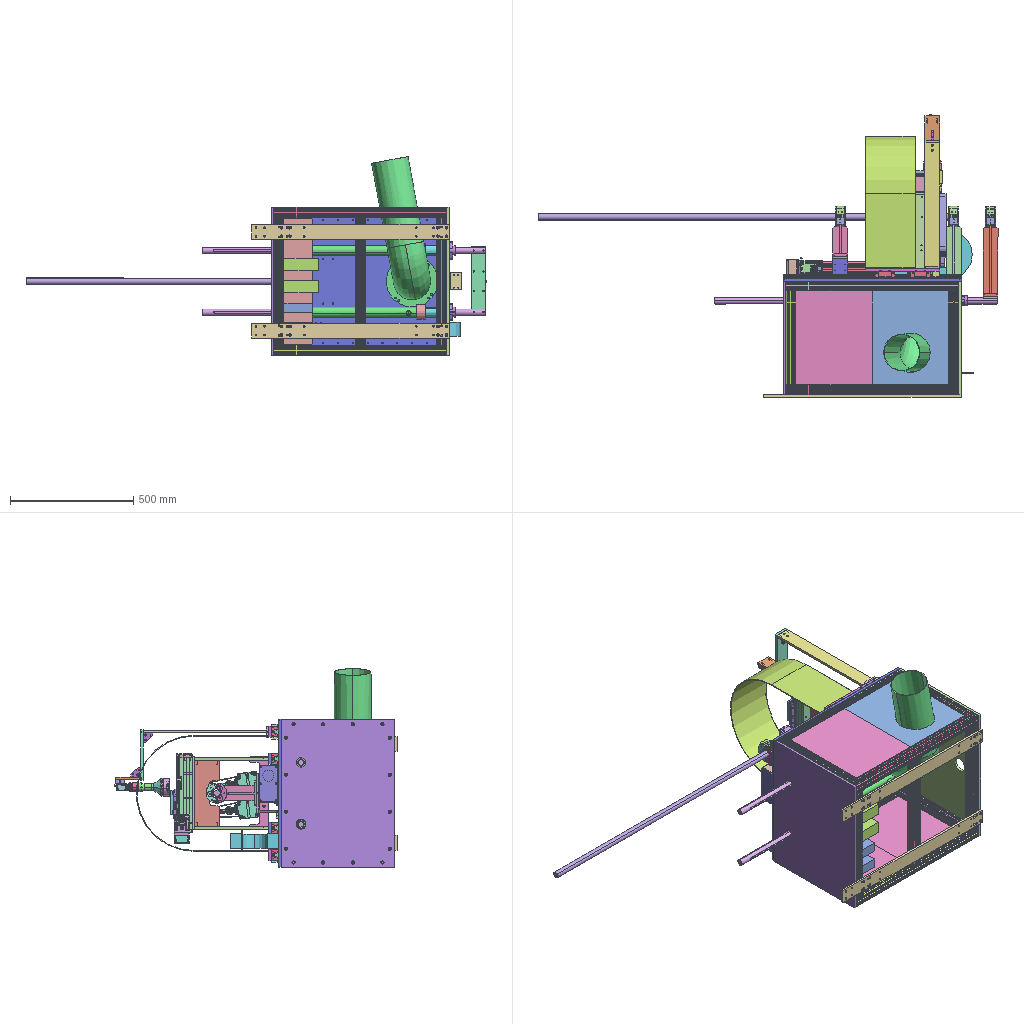Assembly | STEP file | 103 different items | 210 placed | box 1864 x 1144 x 805 mm
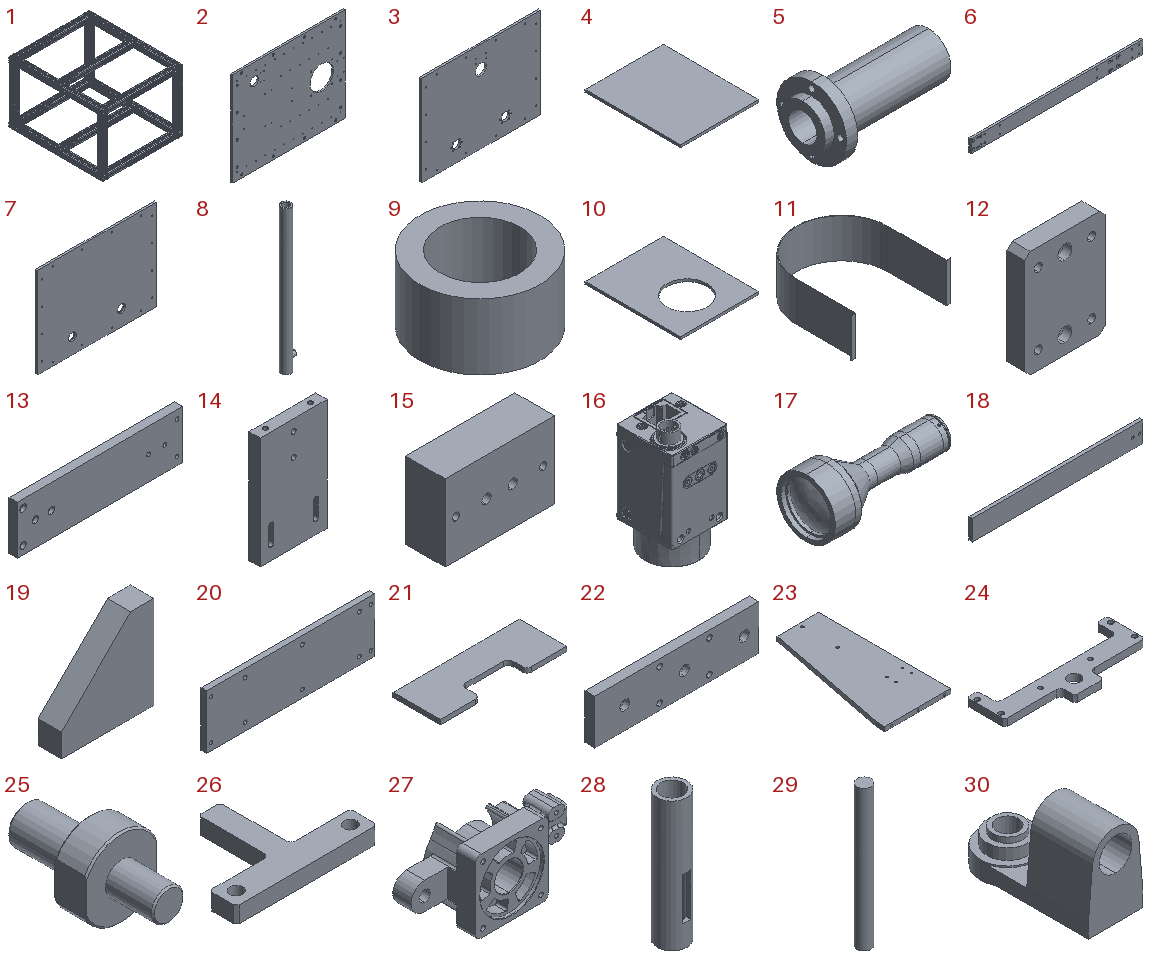Parts list (item | name | quantity | parent item | size | volume):
1 | Grinding bracket-unit 2_Default<machined> | x1 | in 打磨工作台二 | 600 x 700 x 460 mm | 3532999 mm3
2 | Bracket二台Face Plate | x1 | in 打磨工作台二 | 720 x 10 x 600 mm | 4099998 mm3
3 | Bracket二前立Plate | x1 | in 打磨工作台二 | 600 x 10 x 460 mm | 2701010 mm3
4 | 机台DoorPlate-单元二 | x3 | in 打磨工作台二 | 310 x 380 x 10 mm | 1178000 mm3
5 | Linear bearing LMFP25LUU | x2 | in 打磨工作台二 | 112 x 62 x 62 mm | 101190 mm3
6 | 打磨单元二底Plate | x2 | in 打磨工作台二 | 800 x 10 x 60 mm | 468480 mm3
7 | Bracket二后立Plate | x1 | in 打磨工作台二 | 600 x 10 x 460 mm | 2728752 mm3
8 | Aluminium alloy sleeve | x2 | in 打磨工作台二 | 55 x 40 x 600 mm | 439299 mm3
9 | Shaft retaining ring | x2 | in 打磨工作台二 | 60 x 60 x 33 mm | 51836 mm3
10 | 机台DoorPlate开Hole-单元二 | x1 | in 打磨工作台二 | 310 x 380 x 10 mm | 976938 mm3
11 | Dust cover | x1 | - | 510 x 538 x 200 mm | 827737 mm3
12 | Camera bracket base plate | x1 | in Camera bracket | 45 x 10 x 60 mm | 25550 mm3
13 | Camera bracket top plate | x1 | in Camera bracket | 205 x 10 x 60 mm | 120463 mm3
14 | Camera mounting upright plate | x1 | in Camera mounting assembly | 60 x 10 x 100 mm | 50291 mm3
15 | Camera connecting plate | x1 | in Camera mounting assembly | 50 x 18 x 35 mm | 30828 mm3
16 | Basler ace GigE C-Mount v01(1) | x1 | in Camera & lens | 29 x 29.002 x 60.3 mm | 34730 mm3
17 | XF-10MDT04X110-1C | x1 | in Camera & lens | - | -
18 | Camera bracket upright plate | x1 | in Camera bracket | 500 x 10 x 60 mm | 298858 mm3
19 | Camera bracket reinforcement plate | x2 | in Camera bracket | 40 x 10 x 40 mm | 11008 mm3
20 | Grinding bracket top plate | x1 | in Grinding sliding bracket | 295 x 10 x 95 mm | 275998 mm3
21 | Grinding bracket middle plate | x1 | in Grinding sliding bracket | 270 x 100 x 10 mm | 229012 mm3
22 | Grinding bracket base plate | x2 | in Grinding sliding bracket | 165 x 10 x 45 mm | 70401 mm3
23 | Grinding bracket upright plate | x2 | in Grinding sliding bracket | 150 x 300 x 10 mm | 370376 mm3
24 | Polisher mounting plate | x1 | in Grinding sliding bracket | 295 x 110 x 15 mm | 210947 mm3
25 | Polisher lower hinge | x2 | in Grinding sliding bracket | 22 x 45 x 25 mm | 7723 mm3
26 | Polisher shift lever | x1 | in Sliding grinding assembly | 130 x 90 x 15 mm | 64737 mm3
27 | Belt polisher base | x2 | in Polisher | 170 x 58 x 80 mm | 200572 mm3
28 | Polisher lead screw | x2 | in Polisher | 16 x 16 x 70 mm | 5755 mm3
29 | Sliding rod | x2 | in Polisher | 12 x 12 x 120 mm | 13572 mm3
30 | Polisher L bracket | x2 | in Polisher | 20 x 49.5 x 31.5 mm | 12628 mm3
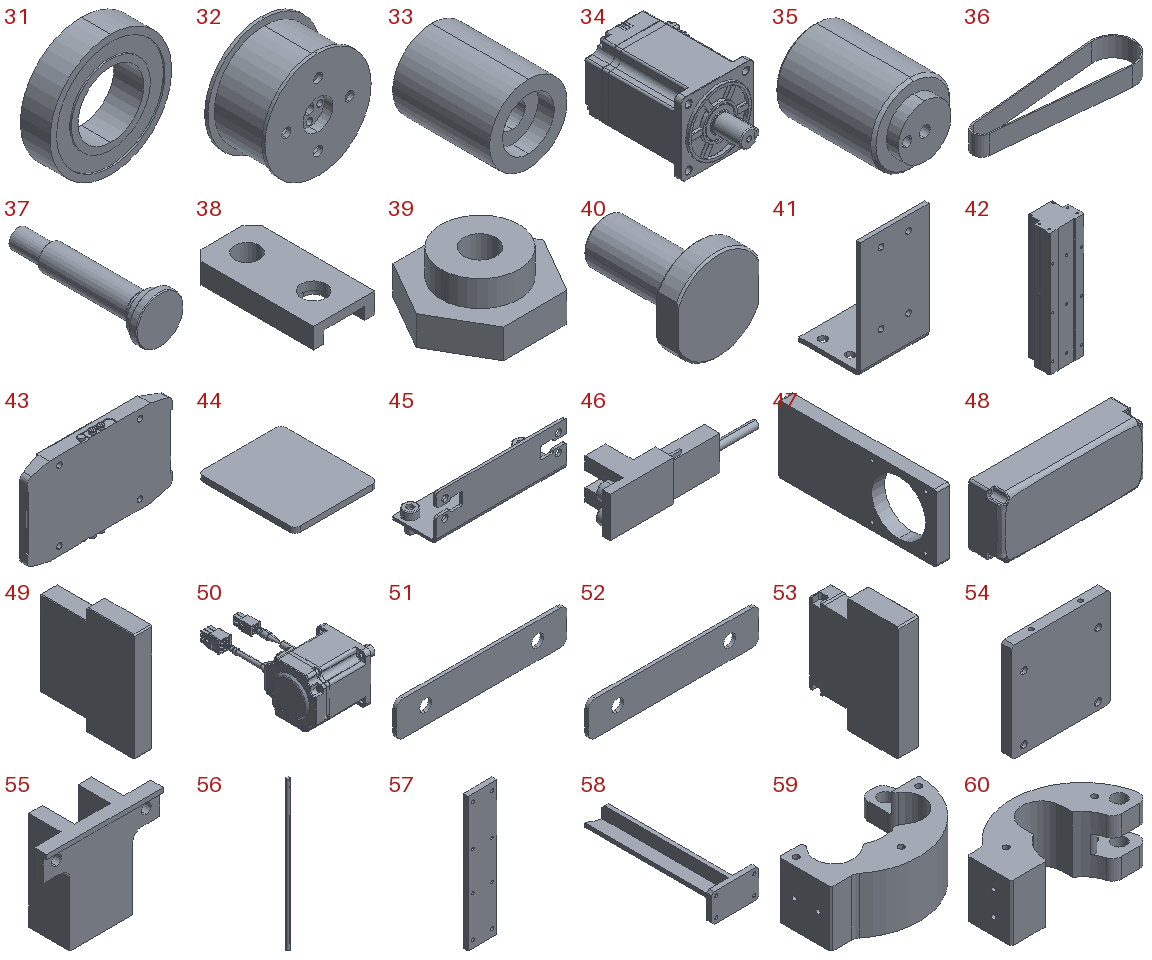31 | Bearing 6904 | x2 | in Polisher | 37 x 9 x 37 mm | 6447 mm3
32 | Polisher large pulley | x2 | in Polisher | 71 x 36 x 71 mm | 28167 mm3
33 | Polisher small pulley | x2 | in Polisher | 24 x 30 x 24 mm | 10556 mm3
34 | 01113977-WXSTEP_B01_整机3D模型_MS1H4-75B30CB-T331R | x2 | in Polisher | - | -
35 | Rotating shaft | x2 | in Polisher | 30 x 42 x 30 mm | 17511 mm3
36 | Sander belt | x2 | in Polisher | 254.5 x 67 x 30 mm | 33527 mm3
37 | Small pulley shaft | x2 | in Polisher | 15 x 45 x 15 mm | 2496 mm3
38 | Polisher connecting part | x2 | in Polisher | 30 x 60 x 10 mm | 13231 mm3
39 | Small pulley nut | x2 | in Polisher | 19.63 x 17 x 8.5 mm | 1412 mm3
40 | Polisher upper hinge | x2 | in Polisher | 22 x 31 x 25 mm | 5247 mm3
41 | 3038 drag chain bracket | x1 | in Sliding grinding assembly | 50 x 45 x 85 mm | 18400 mm3
42 | - | x1 | in GTH8-BL-200W-100L.STEP | 82 x 64 x 290 mm | 1277181 mm3
43 | - | x1 | in GTH8-BL-200W-100L.STEP | - | -
44 | - | x2 | in GTH8-BL-200W-100L.STEP | 15 x 17.5 x 1 mm | 261.642 mm3
45 | - | x3 | in GTH8-BL-200W-100L.STEP | 52.5 x 18 x 23 mm | 1898 mm3
46 | - | x3 | in GTH8-BL-200W-100L.STEP | 52.5 x 15.5 x 13.6 mm | 3264 mm3
47 | - | x1 | in GTH8-BL-200W-100L.STEP | 12 x 146 x 62 mm | 84618 mm3
48 | - | x1 | in GTH8-BL-200W-100L.STEP | - | 40401 mm3
49 | - | x1 | in GTH8-BL-200W-100L.STEP | 13 x 72 x 82 mm | 68483 mm3
50 | - | x1 | in GTH8-BL-200W-100L.STEP | - | -
51 | - | x1 | in GTH8-BL-200W-100L.STEP | 49.5 x 1 x 10 mm | 472.324 mm3
52 | - | x1 | in GTH8-BL-200W-100L.STEP | 49.5 x 1 x 10 mm | 472.324 mm3
53 | - | x1 | in GTH8-BL-200W-100L.STEP | 15 x 63 x 81 mm | 65609 mm3
54 | Slide table mounting plate | x1 | in GTH8-BL-200W-100L | 100 x 10 x 100 mm | 96358 mm3
55 | Sliding fork | x1 | in GTH8-BL-200W-100L | 65 x 25 x 55 mm | 26866 mm3
56 | Extension support shaft | x2 | in Extension support assembly | 25 x 25 x 1150 mm | 526631 mm3
57 | Movable tube support mount | x1 | in Extension support assembly | 60 x 10 x 280 mm | 165846 mm3
58 | Tube support base-extension | x1 | in Tube support assembly-extension section | 100 x 288 x 60 mm | 299980 mm3
59 | Support intermediate piece-lower | x3 | in Support cylinder assembly | 80 x 58 x 32 mm | 47494 mm3
60 | Support intermediate piece-upper | x3 | in Support cylinder assembly | 79.293 x 40 x 32 mm | 45814 mm3
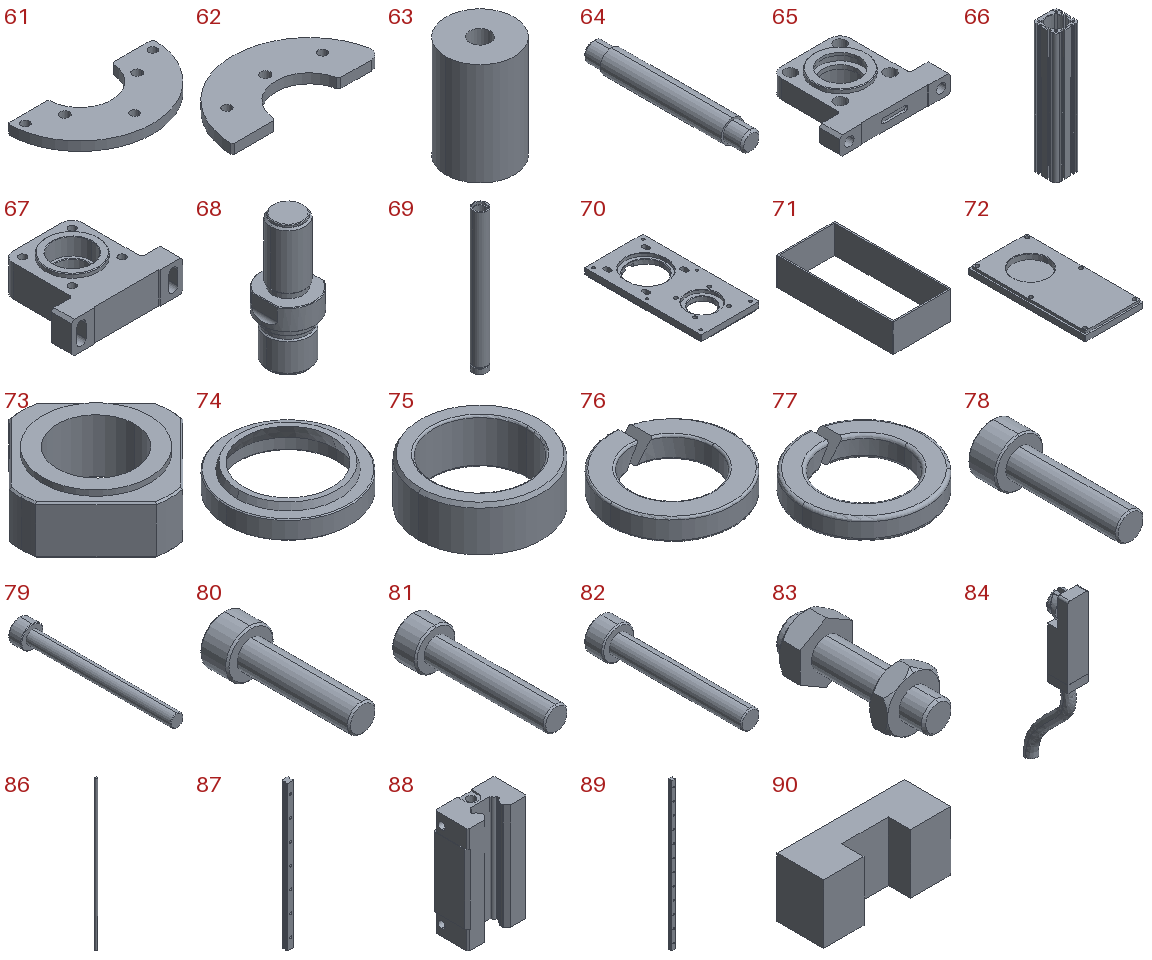61 | End cover plate-lower | x6 | in Support cylinder assembly | 79.976 x 40 x 5 mm | 9716 mm3
62 | End cover plate-upper | x6 | in Support cylinder assembly | 79.281 x 40 x 5 mm | 9633 mm3
63 | Polyurethane roller ABA-2030-686-6 | x9 | in Support cylinder assembly | 20 x 20 x 30 mm | 8577 mm3
64 | Polyurethane roller shaft | x9 | in Support cylinder assembly | 6 x 42 x 6 mm | 1097 mm3
65 | 01前Flange EDA50-L_R04-001-BZ^EDA50-R04 (D60N) | x1 | in EDA50-R04 (D60N) | 85 x 68.5 x 22 mm | 45727 mm3
66 | 03缸体 EDA50-L_R-003-BZ^EDA50-R04 (D60N) | x1 | in EDA50-R04 (D60N) | 53 x 53 x 287 mm | 312692 mm3
67 | 04轴承座 EDA50-L_R04-004-BZ^EDA50-R04 (D60N) | x1 | in EDA50-R04 (D60N) | 85 x 68.5 x 30 mm | 78011 mm3
68 | 05螺纹接头 EDA50-L_R-005-BZ^EDA50-R04 (D60N) | x1 | in EDA50-R04 (D60N) | 25 x 25 x 60 mm | 16821 mm3
69 | 06活塞杆 EDA50-L_R-006-BZ^EDA50-R04 (D60N) | x1 | in EDA50-R04 (D60N) | 25 x 25 x 250 mm | 75291 mm3
70 | 10电机Plate EDA50-R-010-D60NH-BZ^EDA50-R04 (D60N) | x1 | in EDA50-R04 (D60N) | 75 x 150 x 10 mm | 76605 mm3
71 | 11 Timing Pulley盒 EDA50-R-011-BZ^EDA50-R04 (D60N) | x1 | in EDA50-R04 (D60N) | 75 x 150 x 36 mm | 31793 mm3
72 | 12底Plate EDA50-R-012-BZ^EDA50-R04 (D60N) | x1 | in EDA50-R04 (D60N) | 75 x 150 x 10 mm | 96841 mm3
73 | Square precision nut RN_M16×1.5P | x1 | in EDA50-R04 (D60N) | 28 x 28 x 10 mm | 3186 mm3
74 | Dust seal DHS25×33×4.5 | x1 | in EDA50-R04 (D60N) | 33 x 33 x 6.667 mm | 1830 mm3
75 | Graphite bronze bushing JDB253312 | x1 | in EDA50-R04 (D60N) | 33 x 33 x 12 mm | 4332 mm3
76 | 弹垫-4^EDA50-R04 (D60N) | x4 | in EDA50-R04 (D60N) | 6.3 x 6.3 x 1.1 mm | 18.959 mm3
77 | 弹垫-5^EDA50-R04 (D60N) | x12 | in EDA50-R04 (D60N) | 7.7 x 7.7 x 1.3 mm | 32.202 mm3
78 | Hex socket screw M4×16 | x4 | in EDA50-R04 (D60N) | 7 x 20 x 7 mm | 336.359 mm3
79 | Hex socket screw M4×45 | x6 | in EDA50-R04 (D60N) | 7 x 49 x 7 mm | 700.783 mm3
80 | Hex socket screw M5×20 | x4 | in EDA50-R04 (D60N) | 8.5 x 25 x 8.5 mm | 630.064 mm3
81 | Hex socket screw M5×25 | x4 | in EDA50-R04 (D60N) | 8.5 x 30 x 8.5 mm | 728.239 mm3
82 | Hex socket screw M5×35 | x4 | in EDA50-R04 (D60N) | 8.5 x 40 x 8.5 mm | 924.588 mm3
83 | Shoulder stop bolt M4×20 | x1 | in EDA50-R04 (D60N) | 7 x 19.3 x 8.083 mm | 405.674 mm3
84 | Magnetic sensor switch DGN | x3 | in EDA50-R04 (D60N) | 6.2 x 12.865 x 39.622 mm | 580.439 mm3
85 | 0.4KW 60N-14 V7E-L06A-R4030-□1^EDA50-R04 (D60N) | x1 | in EDA50-R04 (D60N) | - | -
86 | 管-1700 | x1 | - | 25.4 x 25.4 x 1700 mm | 861403 mm3
87 | HGR20_3_AF0_1 | x2 | in HGH20CA | 20 x 17.5 x 420 mm | 118454 mm3
88 | HGH20_3_AF0_1 | x6 | in HGH20CA, HGH20CA inspection rail assembly | 44 x 25.4 x 77.5 mm | 65768 mm3
89 | HGR20_3_AF0_1-700 | x2 | in HGH20CA inspection rail assembly | 20 x 17.5 x 720 mm | 203064 mm3
90 | Clamp-HGH20 | x2 | in HGH20CA inspection rail assembly | 60 x 22 x 28 mm | 29915 mm3
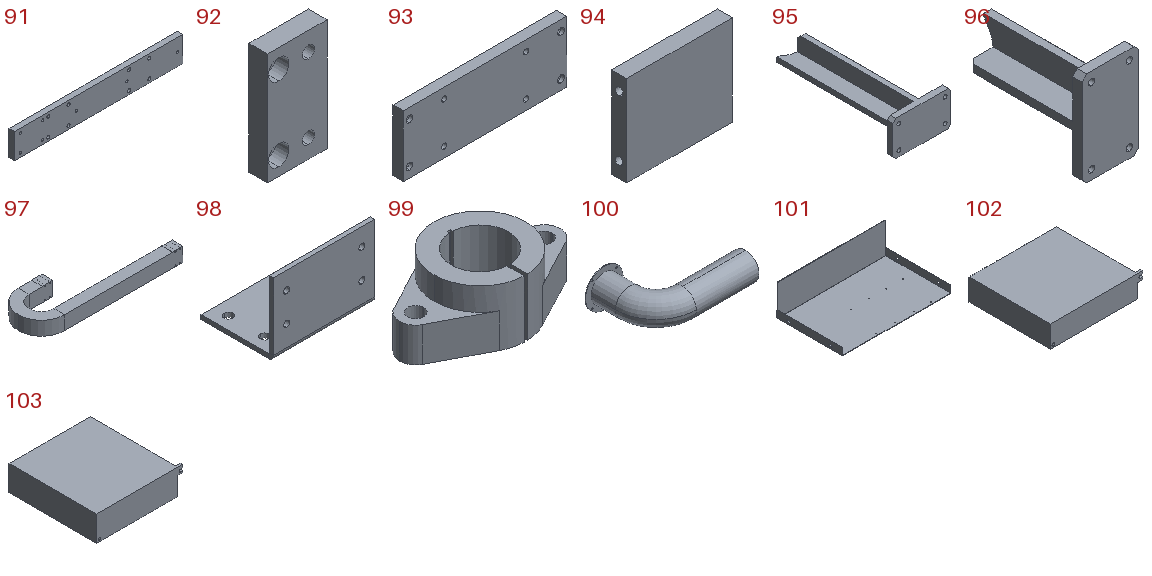91 | Dust cover sliding base plate | x2 | - | 300 x 10 x 45 mm | 129631 mm3
92 | Tube support mounting bracket base plate | x2 | in Tube support mounting bracket | 32 x 10 x 60 mm | 17004 mm3
93 | Tube support mounting bracket top plate | x1 | in Tube support mounting bracket | 160 x 10 x 60 mm | 92192 mm3
94 | Tube support mounting bracket upright plate | x2 | in Tube support mounting bracket | 70 x 10 x 60 mm | 40154 mm3
95 | Tube support base-front end | x1 | in Tube support assembly-front end | 100 x 220 x 60 mm | 239052 mm3
96 | Tube support base-rear end | x1 | in Tube support assembly-rear end | 60 x 130 x 100 mm | 158412 mm3
97 | Drag chain 3038 | x1 | - | 597.5 x 195 x 60 mm | 2179375 mm3
98 | 3050 drag chain bracket | x1 | - | 70 x 50 x 50 mm | 19663 mm3
99 | Open retaining ring | x2 | - | 70 x 39.986 x 25 mm | 26299 mm3
100 | Exhaust duct | x1 | - | 605 x 365 x 210 mm | 724892 mm3
101 | 工作台二电气安装Plate | x1 | in 工作台二电气安装Component | 518 x 310 x 150 mm | 510899 mm3
102 | Jiemeikang 400W driver | x2 | in 工作台二电气安装Component | 170 x 150 x 40 mm | 960193 mm3
103 | Jiemeikang 750W driver | x2 | in 工作台二电气安装Component | 170 x 173 x 50 mm | 1384193 mm3
Placements (level | parent | child | x y z in mm | rotation matrix by rows):
1 | subassembly 2 | 打磨工作台二 | -0.0 -0.0 -0.0 | 0 -1 0 0 0 1 -1 0 0
2 | 打磨工作台二 | Grinding bracket-unit 2_Default<machined> | -0.0 -0.0 -0.0 | 1 0 0 0 1 0 0 0 1
2 | 打磨工作台二 | Bracket二台Face Plate | -0.0 -0.0 450.0 | 0 0 1 -1 0 0 0 -1 0
2 | 打磨工作台二 | Bracket二前立Plate | 0.0 -360.0 210.0 | -1 0 0 0 1 0 0 0 -1
2 | 打磨工作台二 | 机台DoorPlate-单元二 | 290.0 -155.0 210.0 | 0 0 1 -1 0 0 0 -1 0
2 | 打磨工作台二 | 机台DoorPlate-单元二 | 290.0 155.0 210.0 | 0 0 1 -1 0 0 0 -1 0
2 | 打磨工作台二 | 机台DoorPlate-单元二 | -300.0 155.0 210.0 | 0 0 1 -1 0 0 0 -1 0
2 | 打磨工作台二 | Linear bearing LMFP25LUU | -125.0 -350.0 360.0 | 0 -0.7071 -0.7071 1 0 0 0 -0.7071 0.7071
2 | 打磨工作台二 | Linear bearing LMFP25LUU | 125.0 -350.0 360.0 | 0 -0.7071 0.7071 1 0 0 0 0.7071 0.7071
2 | 打磨工作台二 | 打磨单元二底Plate | -200.0 -0.0 -30.0 | 0 0 1 1 0 0 0 1 0
2 | 打磨工作台二 | 打磨单元二底Plate | 200.0 0.0 -30.0 | 0 0 1 1 0 0 0 1 0
2 | 打磨工作台二 | Bracket二后立Plate | -0.0 350.0 210.0 | -1 0 0 0 1 0 0 0 -1
2 | 打磨工作台二 | Aluminium alloy sleeve | 125.0 54.0 360.0 | 0.1874 -0.9823 0 0 0 1 -0.9823 -0.1874 0
2 | 打磨工作台二 | Aluminium alloy sleeve | -125.0 54.0 360.0 | 0.32 -0.9474 0 0 0 1 -0.9474 -0.32 0
2 | 打磨工作台二 | Shaft retaining ring | -125.0 -246.0 360.0 | 0.9187 -0.3949 0 0 0 -1 0.3949 0.9187 -0
2 | 打磨工作台二 | Shaft retaining ring | 125.0 -246.0 360.0 | 1 0 0 0 0 1 0 -1 0
2 | 打磨工作台二 | 机台DoorPlate开Hole-单元二 | -290.0 -155.0 210.0 | 0 0 -1 -1 0 0 0 1 0
1 | subassembly 2 | Dust cover | 73.527 793.0 -0.0 | 0 0 1 0 1 0 -1 0 -0
1 | subassembly 2 | Camera bracket | 243.527 490.0 250.0 | 0 0 -1 0 1 0 1 0 -0
2 | Camera bracket | Camera bracket base plate | -0.0 -0.0 -0.0 | 1 0 0 0 1 0 0 0 1
2 | Camera bracket | Camera bracket top plate | -95.0 510.0 -0.0 | 1 0 0 0 1 0 0 0 1
2 | Camera bracket | Camera mounting assembly | -201.523 570.0 81.376 | 0 -1 0 0 0 -1 1 0 0
3 | Camera mounting assembly | Camera mounting upright plate | -81.376 -16.523 -0.0 | 1 0 0 0 1 0 0 0 1
3 | Camera mounting assembly | Camera connecting plate | -81.376 -0.0229 -50.0 | 1 0 0 0 1 0 0 0 1
3 | Camera mounting assembly | Camera & lens | -81.376 23.477 6.0 | -1 0 0 0 1 0 0 0 -1
4 | Camera & lens | Basler ace GigE C-Mount v01(1) | -0.0 -0.0 -0.0 | 1 0 0 0 1 0 0 0 1
4 | Camera & lens | XF-10MDT04X110-1C | -0.0 -0.0 -161.27 | 0 0.1355 -0.9908 0 0.9908 0.1355 1 0 0
2 | Camera bracket | Camera bracket upright plate | 5.0 260.0 -0.0 | 0 -1 0 1 0 0 0 0 1
2 | Camera bracket | Camera bracket reinforcement plate | -25.0 490.0 -5.0 | 1 0 0 0 0 -1 0 1 0
2 | Camera bracket | Camera bracket reinforcement plate | -165.0 540.0 5.0 | 0 0 1 -1 0 0 0 -1 0
1 | subassembly 2 | Sliding grinding assembly | 202.0 480.0 -0.0 | 0 0 1 0 1 0 -1 0 0
2 | Sliding grinding assembly | Grinding sliding bracket | -0.0 -0.0 -0.0 | 1 0 0 0 1 0 0 0 1
3 | Grinding sliding bracket | Grinding bracket top plate | -0.0 310.0 -0.0 | 1 0 0 0 1 0 0 0 1
3 | Grinding sliding bracket | Grinding bracket middle plate | -0.0 260.0 -0.0 | 1 0 0 0 1 0 0 0 1
3 | Grinding sliding bracket | Grinding bracket base plate | -140.0 -0.0 -27.5 | 0 0 1 0 1 0 -1 0 0
3 | Grinding sliding bracket | Grinding bracket base plate | 140.0 -0.0 -27.5 | 0 0 1 0 1 0 -1 0 0
3 | Grinding sliding bracket | Grinding bracket upright plate | -135.0 160.0 -27.5 | 0 0 -1 0 1 0 1 0 0
3 | Grinding sliding bracket | Grinding bracket upright plate | 145.0 160.0 -27.5 | 0 0 -1 0 1 0 1 0 0
3 | Grinding sliding bracket | Polisher mounting plate | 0.0 50.0 55.0 | 1 0 0 0 1 0 0 0 1
3 | Grinding sliding bracket | Polisher lower hinge | -52.5 30.0 47.5 | -0.9237 0 -0.383 -0.383 0 0.9237 0 1 -0
3 | Grinding sliding bracket | Polisher lower hinge | 52.5 30.0 47.5 | -0.9237 0 -0.383 -0.383 0 0.9237 0 1 -0
2 | Sliding grinding assembly | Polisher shift lever | 37.5 332.182 65.5 | 1 0 0 0 1 0 0 0 1
2 | Sliding grinding assembly | Polisher | 60.505 94.505 54.5 | 0.1232 0 0.9924 0.9924 0 -0.1232 0 1 -0
3 | Polisher | Belt polisher base | -0.0 0.0 -0.0 | 1 0 0 0 1 0 0 0 1
3 | Polisher | Polisher lead screw | 95.0 28.0 -0.0 | 0 0 -1 1 0 0 0 -1 0
3 | Polisher | Sliding rod | 130.0 28.0 -0.0 | 0 0 1 0.7951 0.6065 0 -0.6065 0.7951 0
3 | Polisher | Polisher L bracket | 167.5 28.0 -0.0 | 0 1 0 0 0 1 1 0 -0
3 | Polisher | Bearing 6904 | -0.0 32.5 -0.0 | 1 0 0 0 1 0 0 0 1
3 | Polisher | Polisher large pulley | -0.0 26.5 -0.0 | -0.916 0 -0.4012 0 -1 0 -0.4012 0 0.916
3 | Polisher | Polisher small pulley | 207.0 27.5 -0.0 | 0.09008 0 -0.9959 0 -1 0 -0.9959 0 -0.09008
3 | Polisher | 01113977-WXSTEP_B01_整机3D模型_MS1H4-75B30CB-T331R | -40.169 -9.999 -40.169 | 1 0 0 0 -1 0 0 0 -1
3 | Polisher | Rotating shaft | -0.0 32.5 -0.0 | -0.8372 0 -0.5469 0 -1 0 -0.5469 0 0.8372
3 | Polisher | Sander belt | 103.5 27.5 -0.0 | -1 0 0 0 0 -1 0 -1 0
3 | Polisher | Small pulley shaft | 207.0 42.5 -0.0 | -0.4626 0 -0.8865 0 -1 0 -0.8865 0 0.4626
3 | Polisher | Polisher connecting part | 192.0 11.0 -0.0 | 0 1 0 0 0 -1 -1 0 0
3 | Polisher | Small pulley nut | 207.0 -3.5 -0.0 | 0.9774 -0.2115 0 0 0 1 -0.2115 -0.9774 -0
3 | Polisher | Polisher upper hinge | 239.5 -5.0 -0.0 | 0.9999 0 0.01272 0 1 0 -0.01272 0 0.9999
2 | Sliding grinding assembly | Polisher | -44.495 94.505 54.5 | 0.1232 0 0.9924 0.9924 0 -0.1232 0 1 0
3 | Polisher | Belt polisher base | -0.0 0.0 -0.0 | 1 0 0 0 1 0 0 0 1
3 | Polisher | Polisher lead screw | 95.0 28.0 -0.0 | 0 0 -1 1 0 0 0 -1 0
3 | Polisher | Sliding rod | 130.0 28.0 -0.0 | 0 0 1 0.7951 0.6065 0 -0.6065 0.7951 0
3 | Polisher | Polisher L bracket | 167.5 28.0 -0.0 | 0 1 0 0 0 1 1 0 -0
3 | Polisher | Bearing 6904 | -0.0 32.5 -0.0 | 1 0 0 0 1 0 0 0 1
3 | Polisher | Polisher large pulley | -0.0 26.5 -0.0 | -0.916 0 -0.4012 0 -1 0 -0.4012 0 0.916
3 | Polisher | Polisher small pulley | 207.0 27.5 -0.0 | 0.09008 0 -0.9959 0 -1 0 -0.9959 0 -0.09008
3 | Polisher | 01113977-WXSTEP_B01_整机3D模型_MS1H4-75B30CB-T331R | -40.169 -9.999 -40.169 | 1 0 0 0 -1 0 0 0 -1
3 | Polisher | Rotating shaft | -0.0 32.5 -0.0 | -0.8372 0 -0.5469 0 -1 0 -0.5469 0 0.8372
3 | Polisher | Sander belt | 103.5 27.5 -0.0 | -1 0 0 0 0 -1 0 -1 0
3 | Polisher | Small pulley shaft | 207.0 42.5 -0.0 | -0.4626 0 -0.8865 0 -1 0 -0.8865 0 0.4626
3 | Polisher | Polisher connecting part | 192.0 11.0 -0.0 | 0 1 0 0 0 -1 -1 0 0
3 | Polisher | Small pulley nut | 207.0 -3.5 -0.0 | 0.9774 -0.2115 0 0 0 1 -0.2115 -0.9774 -0
3 | Polisher | Polisher upper hinge | 239.5 -5.0 -0.0 | 0.9999 0 0.01272 0 1 0 -0.01272 0 0.9999
2 | Sliding grinding assembly | 3038 drag chain bracket | 187.5 117.0 15.0 | 0 0 1 0 -1 0 1 0 -0
2 | Sliding grinding assembly | GTH8-BL-200W-100L | -0.0 320.0 -0.0 | -1 0 0 0 1 0 0 0 -1
3 | GTH8-BL-200W-100L | GTH8-BL-200W-100L.STEP | -145.0 -0.0 -0.0 | 1 0 0 0 1 0 0 0 1
4 | GTH8-BL-200W-100L.STEP | subassembly 3 | 0.0 0.0 0.0 | 0 0 1 0 1 0 -1 0 -0
4 | GTH8-BL-200W-100L.STEP | subassembly 4 | 94.3 65.0 -0.0 | 1 0 0 0 1 0 0 0 1
4 | GTH8-BL-200W-100L.STEP | subassembly 5 | 94.3 63.0 0.8 | -1 0 0 0 -1 0 0 0 1
4 | GTH8-BL-200W-100L.STEP | subassembly 5 | 94.3 63.0 -0.8 | 1 0 0 0 -1 0 0 0 -1
4 | GTH8-BL-200W-100L.STEP | subassembly 6 | 159.95 44.5 28.5 | 1 0 0 0 1 0 0 0 1
4 | GTH8-BL-200W-100L.STEP | subassembly 7 | 212.45 45.5 39.5 | -1 0 0 0 1 0 0 0 -1
4 | GTH8-BL-200W-100L.STEP | subassembly 6 | 94.3 44.5 -28.5 | -1 0 0 0 1 0 0 0 -1
4 | GTH8-BL-200W-100L.STEP | subassembly 7 | 94.3 45.5 -39.5 | -1 0 0 0 1 0 0 0 -1
4 | GTH8-BL-200W-100L.STEP | subassembly 8 | 0.0 43.3 42.4 | 1 0 0 0 0 -1 0 1 0
4 | GTH8-BL-200W-100L.STEP | subassembly 7 | 94.3 45.5 -39.5 | 1 0 0 0 1 0 0 0 1
4 | GTH8-BL-200W-100L.STEP | subassembly 6 | 146.8 44.5 -28.5 | -1 0 0 0 1 0 0 0 -1
4 | GTH8-BL-200W-100L.STEP | subassembly 9 | -58.0 43.3 41.9 | 0 1 0 0 0 1 1 0 -0
4 | GTH8-BL-200W-100L.STEP | subassembly 10 | 0.0 -0.1 -0.0 | 1 0 0 0 1 0 0 0 1
4 | GTH8-BL-200W-100L.STEP | subassembly 11 | -13.0 43.3 80.9 | -1 0 0 0 0 1 0 1 -0
4 | GTH8-BL-200W-100L.STEP | subassembly 12 | 285.0 63.68 0.0 | 0 0 1 0 1 0 -1 0 -0
4 | GTH8-BL-200W-100L.STEP | subassembly 13 | 5.0 63.68 -0.0 | 0 0 1 0 1 0 -1 0 -0
4 | GTH8-BL-200W-100L.STEP | subassembly 14 | 290.0 -0.0 -0.0 | 1 0 0 0 1 0 0 0 1
3 | GTH8-BL-200W-100L | Slide table mounting plate | -37.5 78.0 0.0 | -1 0 0 0 1 0 0 0 -1
3 | GTH8-BL-200W-100L | Sliding fork | -37.5 63.0 -71.5 | 1 0 0 0 0 1 0 -1 -0
1 | subassembly 2 | Extension support assembly | -65.475 360.0 -0.0 | -1 0 0 0 1 0 0 0 -1
2 | Extension support assembly | Extension support shaft | 0.0 0.0 -125.0 | 0 0 -1 0 1 0 1 0 -0
2 | Extension support assembly | Extension support shaft | 0.0 0.0 125.0 | 0 0 -1 0 1 0 1 0 -0
2 | Extension support assembly | Movable tube support mount | -545.0 9.5 0.0 | 1 0 0 0 1 0 0 0 1
2 | Extension support assembly | Tube support assembly-extension section | -545.0 19.5 0.0 | 0 0 -1 0 1 0 1 0 -0
3 | Tube support assembly-extension section | Tube support base-extension | -0.0 -0.0 -0.0 | 1 0 0 0 1 0 0 0 1
3 | Tube support assembly-extension section | Support cylinder assembly | -0.0 318.0 -0.0 | 1 0 0 0 1 0 0 0 1
4 | Support cylinder assembly | Support intermediate piece-lower | 0.0 0.0 -0.0 | 1 0 0 0 1 0 0 0 1
4 | Support cylinder assembly | Support intermediate piece-upper | -1.093 4.431 -0.0 | 0.9902 0.1398 0 -0.1398 0.9902 0 0 0 1
4 | Support cylinder assembly | End cover plate-lower | 0.0 0.0 16.0 | 1 0 0 0 1 0 0 0 1
4 | Support cylinder assembly | End cover plate-lower | 0.0 0.0 -16.0 | -1 0 0 0 1 0 0 0 -1
4 | Support cylinder assembly | End cover plate-upper | -1.093 4.431 16.0 | 0.9902 0.1398 0 -0.1398 0.9902 0 0 0 1
4 | Support cylinder assembly | End cover plate-upper | -1.093 4.431 -21.0 | 0.9902 0.1398 0 -0.1398 0.9902 0 0 0 1
4 | Support cylinder assembly | Polyurethane roller ABA-2030-686-6 | -19.919 -11.5 -0.0 | 1 0 0 0 1 0 0 0 1
4 | Support cylinder assembly | Polyurethane roller shaft | -19.919 -11.5 0.0 | 0.6705 0 -0.7419 -0.7419 0 -0.6705 0 1 0
4 | Support cylinder assembly | Polyurethane roller shaft | 19.919 -11.5 0.0 | 0.5134 0 -0.8581 -0.8581 0 -0.5134 0 1 0
4 | Support cylinder assembly | Polyurethane roller shaft | 2.122 27.206 0.0 | 0.6705 0 -0.7419 -0.7419 0 -0.6705 0 1 0
4 | Support cylinder assembly | Polyurethane roller ABA-2030-686-6 | 19.919 -11.5 -0.0 | 1 0 0 0 1 0 0 0 1
4 | Support cylinder assembly | Polyurethane roller ABA-2030-686-6 | 2.122 27.206 0.0 | 1 0 0 0 1 0 0 0 1
1 | subassembly 2 | EDA50-R04 (D60N) | -130.5 492.0 0.0 | 0 0 1 0 1 0 -1 0 0
2 | EDA50-R04 (D60N) | 01前Flange EDA50-L_R04-001-BZ^EDA50-R04 (D60N) | -0.0 -0.0 150.5 | 1 0 0 0 1 0 0 0 1
2 | EDA50-R04 (D60N) | 03缸体 EDA50-L_R-003-BZ^EDA50-R04 (D60N) | -0.0 -0.0 -0.0 | 1 0 0 0 1 0 0 0 1
2 | EDA50-R04 (D60N) | 04轴承座 EDA50-L_R04-004-BZ^EDA50-R04 (D60N) | -0.0 -0.0 -155.5 | 1 0 0 0 1 0 0 0 1
2 | EDA50-R04 (D60N) | 05螺纹接头 EDA50-L_R-005-BZ^EDA50-R04 (D60N) | -0.0 -0.0 177.5 | 1 0 0 0 1 0 0 0 1
2 | EDA50-R04 (D60N) | 06活塞杆 EDA50-L_R-006-BZ^EDA50-R04 (D60N) | -0.0 0.0 42.5 | 0 1 0 -1 0 0 0 0 1
2 | EDA50-R04 (D60N) | 10电机Plate EDA50-R-010-D60NH-BZ^EDA50-R04 (D60N) | -0.0 -0.0 -172.5 | 0 -1 0 1 0 0 0 0 1
2 | EDA50-R04 (D60N) | 11 Timing Pulley盒 EDA50-R-011-BZ^EDA50-R04 (D60N) | 0.0 -0.0 -192.5 | 0 -1 0 1 0 0 0 0 1
2 | EDA50-R04 (D60N) | 12底Plate EDA50-R-012-BZ^EDA50-R04 (D60N) | -0.0 -0.0 -212.5 | 0 -1 0 1 0 0 0 0 1
2 | EDA50-R04 (D60N) | Square precision nut RN_M16×1.5P | -0.0 -0.0 186.5 | 1 0 0 0 1 0 0 0 1
2 | EDA50-R04 (D60N) | Dust seal DHS25×33×4.5 | -0.0 -0.0 160.167 | 1 0 0 0 1 0 0 0 1
2 | EDA50-R04 (D60N) | Graphite bronze bushing JDB253312 | -0.0 -0.0 144.5 | 1 0 0 0 1 0 0 0 1
2 | EDA50-R04 (D60N) | 弹垫-4^EDA50-R04 (D60N) | 21.651 12.5 -172.55 | 1 0 0 0 1 0 0 0 1
2 | EDA50-R04 (D60N) | 弹垫-5^EDA50-R04 (D60N) | 19.0 19.0 151.15 | -0.9237 0.383 0 -0.383 -0.9237 0 0 0 1
2 | EDA50-R04 (D60N) | 弹垫-5^EDA50-R04 (D60N) | 19.0 -19.0 151.15 | -0.383 -0.9237 0 0.9237 -0.383 0 0 0 1
2 | EDA50-R04 (D60N) | 弹垫-5^EDA50-R04 (D60N) | -19.0 -19.0 151.15 | 0.9237 -0.383 0 0.383 0.9237 0 0 0 1
2 | EDA50-R04 (D60N) | 弹垫-5^EDA50-R04 (D60N) | -19.0 19.0 151.15 | 0.383 0.9237 0 -0.9237 0.383 0 0 0 1
2 | EDA50-R04 (D60N) | 弹垫-5^EDA50-R04 (D60N) | 19.0 19.0 -161.15 | -1 0 0 0 1 0 0 0 -1
2 | EDA50-R04 (D60N) | 弹垫-5^EDA50-R04 (D60N) | -97.249 24.749 -160.35 | -0.7917 -0.611 0 0.611 -0.7917 0 0 0 1
2 | EDA50-R04 (D60N) | 弹垫-5^EDA50-R04 (D60N) | 19.0 -19.0 -161.15 | 0 1 0 1 0 0 0 0 -1
2 | EDA50-R04 (D60N) | 弹垫-5^EDA50-R04 (D60N) | -19.0 -19.0 -161.15 | 1 0 0 0 -1 0 0 0 -1
2 | EDA50-R04 (D60N) | 弹垫-5^EDA50-R04 (D60N) | -19.0 19.0 -161.15 | 0 -1 0 -1 0 0 0 0 -1
2 | EDA50-R04 (D60N) | Hex socket screw M4×16 | 21.651 12.5 -175.1 | -0.9237 0 0.383 -0.383 0 -0.9237 0 -1 0
2 | EDA50-R04 (D60N) | Hex socket screw M4×45 | 30.0 32.0 -215.0 | 1 0 0 0 0 1 0 -1 0
2 | EDA50-R04 (D60N) | Hex socket screw M5×20 | -97.249 24.749 -157.2 | 0.9674 0 -0.2531 -0.2531 0 -0.9674 0 1 0
2 | EDA50-R04 (D60N) | Hex socket screw M5×25 | 19.0 19.0 154.3 | -0.7349 0 0.6782 0.6782 0 0.7349 0 1 -0
2 | EDA50-R04 (D60N) | Hex socket screw M5×25 | 19.0 -19.0 154.3 | 0.6782 0 0.7349 0.7349 0 -0.6782 0 1 -0
2 | EDA50-R04 (D60N) | Hex socket screw M5×25 | -19.0 -19.0 154.3 | 0.7349 0 -0.6782 -0.6782 0 -0.7349 0 1 -0
2 | EDA50-R04 (D60N) | Hex socket screw M5×25 | -19.0 19.0 154.3 | -0.6782 0 -0.7349 -0.7349 0 0.6782 0 1 -0
2 | EDA50-R04 (D60N) | Hex socket screw M5×35 | 19.0 19.0 -164.3 | -0.9237 0 0.383 -0.383 0 -0.9237 0 -1 0
2 | EDA50-R04 (D60N) | Hex socket screw M5×35 | 19.0 -19.0 -164.3 | -0.383 0 -0.9237 0.9237 0 -0.383 0 -1 0
2 | EDA50-R04 (D60N) | Hex socket screw M5×35 | -19.0 -19.0 -164.3 | 0.9237 0 -0.383 0.383 0 0.9237 0 -1 0
2 | EDA50-R04 (D60N) | Hex socket screw M5×35 | -19.0 19.0 -164.3 | 0.383 0 0.9237 -0.9237 0 0.383 0 -1 0
2 | EDA50-R04 (D60N) | Shoulder stop bolt M4×20 | -0.0 39.6 -157.5 | 1 0 0 0 1 0 0 0 1
2 | EDA50-R04 (D60N) | Magnetic sensor switch DGN | 24.5 9.25 119.8 | 0 1 0 -1 0 0 0 0 1
2 | EDA50-R04 (D60N) | Magnetic sensor switch DGN | 24.5 9.25 -103.8 | 0 1 0 1 0 0 0 0 -1
2 | EDA50-R04 (D60N) | Magnetic sensor switch DGN | 24.5 -9.25 -98.8 | 0 1 0 1 0 0 0 0 -1
2 | EDA50-R04 (D60N) | 弹垫-4^EDA50-R04 (D60N) | -12.5 21.651 -172.55 | 0 -1 0 1 0 0 0 0 1
2 | EDA50-R04 (D60N) | 弹垫-4^EDA50-R04 (D60N) | -21.651 -12.5 -172.55 | -1 0 0 0 -1 0 0 0 1
2 | EDA50-R04 (D60N) | 弹垫-4^EDA50-R04 (D60N) | 12.5 -21.651 -172.55 | 0 1 0 -1 0 0 0 0 1
2 | EDA50-R04 (D60N) | Hex socket screw M4×16 | -12.5 21.651 -175.1 | 0.383 0 0.9237 -0.9237 0 0.383 0 -1 0
2 | EDA50-R04 (D60N) | Hex socket screw M4×16 | -21.651 -12.5 -175.1 | 0.9237 0 -0.383 0.383 0 0.9237 0 -1 0
2 | EDA50-R04 (D60N) | Hex socket screw M4×16 | 12.5 -21.651 -175.1 | -0.383 0 -0.9237 0.9237 0 -0.383 0 -1 0
2 | EDA50-R04 (D60N) | Hex socket screw M4×45 | -39.0 32.0 -215.0 | 1 0 0 0 0 1 0 -1 0
2 | EDA50-R04 (D60N) | Hex socket screw M4×45 | -108.0 32.0 -215.0 | 1 0 0 0 0 1 0 -1 0
2 | EDA50-R04 (D60N) | Hex socket screw M4×45 | 30.0 -32.0 -215.0 | 1 0 0 0 0 1 0 -1 0
2 | EDA50-R04 (D60N) | Hex socket screw M4×45 | -39.0 -32.0 -215.0 | 1 0 0 0 0 1 0 -1 0
2 | EDA50-R04 (D60N) | Hex socket screw M4×45 | -108.0 -32.0 -215.0 | 1 0 0 0 0 1 0 -1 0
2 | EDA50-R04 (D60N) | 0.4KW 60N-14 V7E-L06A-R4030-□1^EDA50-R04 (D60N) | -59.622 -0.3173 -161.466 | 0 1 0 -1 0 0 0 0 1
2 | EDA50-R04 (D60N) | Hex socket screw M5×20 | -47.751 24.749 -157.2 | -0.2531 0 -0.9674 -0.9674 0 0.2531 0 1 0
2 | EDA50-R04 (D60N) | Hex socket screw M5×20 | -47.751 -24.749 -157.2 | -0.9674 0 0.2531 0.2531 0 0.9674 0 1 0
2 | EDA50-R04 (D60N) | Hex socket screw M5×20 | -97.249 -24.749 -157.2 | 0.2531 0 0.9674 0.9674 0 -0.2531 0 1 0
2 | EDA50-R04 (D60N) | 弹垫-5^EDA50-R04 (D60N) | -47.751 24.749 -160.35 | 0.611 -0.7917 0 0.7917 0.611 0 0 0 1
2 | EDA50-R04 (D60N) | 弹垫-5^EDA50-R04 (D60N) | -47.751 -24.749 -160.35 | 0.7917 0.611 0 -0.611 0.7917 0 0 0 1
2 | EDA50-R04 (D60N) | 弹垫-5^EDA50-R04 (D60N) | -97.249 -24.749 -160.35 | -0.611 0.7917 0 -0.7917 -0.611 0 0 0 1
1 | subassembly 2 | 管-1700 | -504.613 700.0 0.3816 | -0.000711 -0.000656 -1 0.6779 -0.7351 0 -0.7351 -0.6779 0.000967
1 | subassembly 2 | HGH20CA | 70.0 467.5 140.0 | 0 0 -1 0 1 0 1 0 0
2 | HGH20CA | HGR20_3_AF0_1 | -0.0 -0.0 -0.0 | 1 0 0 0 1 0 0 0 1
2 | HGH20CA | HGH20_3_AF0_1 | -0.0 -0.0 -111.5 | 1 0 0 0 1 0 0 0 1
1 | subassembly 2 | HGH20CA | 70.0 467.5 -140.0 | 0 0 -1 0 1 0 1 0 0
2 | HGH20CA | HGR20_3_AF0_1 | -0.0 -0.0 -0.0 | 1 0 0 0 1 0 0 0 1
2 | HGH20CA | HGH20_3_AF0_1 | 0.0 -0.0 -111.5 | 1 0 0 0 1 0 0 0 1
1 | subassembly 2 | HGH20CA inspection rail assembly | 0.0 467.5 -250.0 | 0 0 1 0 1 0 -1 0 0
2 | HGH20CA inspection rail assembly | HGR20_3_AF0_1-700 | -0.0 -0.0 -0.0 | 1 0 0 0 1 0 0 0 1
2 | HGH20CA inspection rail assembly | HGH20_3_AF0_1 | -0.0 -0.0 51.527 | 1 0 0 0 1 0 0 0 1
2 | HGH20CA inspection rail assembly | HGH20_3_AF0_1 | -0.0 -0.0 195.527 | 1 0 0 0 1 0 0 0 1
2 | HGH20CA inspection rail assembly | Clamp-HGH20 | -0.0 0.5 258.527 | 1 0 0 0 1 0 0 0 1
1 | subassembly 2 | HGH20CA inspection rail assembly | 0.0 467.5 250.0 | 0 0 1 0 1 0 -1 0 0
2 | HGH20CA inspection rail assembly | HGR20_3_AF0_1-700 | -0.0 -0.0 -0.0 | 1 0 0 0 1 0 0 0 1
2 | HGH20CA inspection rail assembly | HGH20_3_AF0_1 | -0.0 -0.0 51.527 | 1 0 0 0 1 0 0 0 1
2 | HGH20CA inspection rail assembly | HGH20_3_AF0_1 | -0.0 -0.0 195.527 | 1 0 0 0 1 0 0 0 1
2 | HGH20CA inspection rail assembly | Clamp-HGH20 | -0.0 0.5 258.527 | 1 0 0 0 1 0 0 0 1
1 | subassembly 2 | Dust cover sliding base plate | 73.527 480.0 -250.0 | -1 0 0 0 1 0 0 0 -1
1 | subassembly 2 | Dust cover sliding base plate | 73.527 480.0 250.0 | -1 0 0 0 1 0 0 0 -1
1 | subassembly 2 | Tube support mounting bracket | -130.0 450.0 0.0 | 0 0 -1 0 1 0 1 0 0
2 | Tube support mounting bracket | Tube support mounting bracket base plate | 84.0 -0.0 -0.0 | 1 0 0 0 1 0 0 0 1
2 | Tube support mounting bracket | Tube support mounting bracket base plate | -84.0 -0.0 -0.0 | -1 0 0 0 1 0 0 0 -1
2 | Tube support mounting bracket | Tube support mounting bracket top plate | -0.0 80.0 -0.0 | 1 0 0 0 1 0 0 0 1
2 | Tube support mounting bracket | Tube support mounting bracket upright plate | -74.0 45.0 -0.0 | 0 1 0 -1 0 0 0 0 1
2 | Tube support mounting bracket | Tube support mounting bracket upright plate | 74.0 45.0 -0.0 | 0 1 0 -1 0 0 0 0 1
1 | subassembly 2 | Tube support assembly-front end | 330.0 450.0 -0.0 | 0 0 1 0 1 0 -1 0 -0
2 | Tube support assembly-front end | Tube support base-front end | -0.0 -0.0 -0.0 | 1 0 0 0 1 0 0 0 1
2 | Tube support assembly-front end | Support cylinder assembly | -0.0 250.0 -0.0 | 1 0 0 0 1 0 0 0 1
3 | Support cylinder assembly | Support intermediate piece-lower | 0.0 0.0 -0.0 | 1 0 0 0 1 0 0 0 1
3 | Support cylinder assembly | Support intermediate piece-upper | -1.093 4.431 -0.0 | 0.9902 0.1398 0 -0.1398 0.9902 0 0 0 1
3 | Support cylinder assembly | End cover plate-lower | 0.0 0.0 16.0 | 1 0 0 0 1 0 0 0 1
3 | Support cylinder assembly | End cover plate-lower | 0.0 0.0 -16.0 | -1 0 0 0 1 0 0 0 -1
3 | Support cylinder assembly | End cover plate-upper | -1.093 4.431 16.0 | 0.9902 0.1398 0 -0.1398 0.9902 0 0 0 1
3 | Support cylinder assembly | End cover plate-upper | -1.093 4.431 -21.0 | 0.9902 0.1398 0 -0.1398 0.9902 0 0 0 1
3 | Support cylinder assembly | Polyurethane roller ABA-2030-686-6 | -19.919 -11.5 -0.0 | 1 0 0 0 1 0 0 0 1
3 | Support cylinder assembly | Polyurethane roller shaft | -19.919 -11.5 0.0 | 0.6705 0 -0.7419 -0.7419 0 -0.6705 0 1 0
3 | Support cylinder assembly | Polyurethane roller shaft | 19.919 -11.5 0.0 | 0.5134 0 -0.8581 -0.8581 0 -0.5134 0 1 0
3 | Support cylinder assembly | Polyurethane roller shaft | 2.122 27.206 0.0 | 0.6705 0 -0.7419 -0.7419 0 -0.6705 0 1 0
3 | Support cylinder assembly | Polyurethane roller ABA-2030-686-6 | 19.919 -11.5 -0.0 | 1 0 0 0 1 0 0 0 1
3 | Support cylinder assembly | Polyurethane roller ABA-2030-686-6 | 2.122 27.206 0.0 | 1 0 0 0 1 0 0 0 1
1 | subassembly 2 | Tube support assembly-rear end | -130.0 540.0 0.0 | 1 0 0 0 1 0 0 0 1
2 | Tube support assembly-rear end | Tube support base-rear end | -0.0 -0.0 -0.0 | 1 0 0 0 1 0 0 0 1
2 | Tube support assembly-rear end | Support cylinder assembly | -0.0 160.0 -0.0 | 0 0 1 0 1 0 -1 0 0
3 | Support cylinder assembly | Support intermediate piece-lower | 0.0 0.0 -0.0 | 1 0 0 0 1 0 0 0 1
3 | Support cylinder assembly | Support intermediate piece-upper | -1.093 4.431 -0.0 | 0.9902 0.1398 0 -0.1398 0.9902 0 0 0 1
3 | Support cylinder assembly | End cover plate-lower | 0.0 0.0 16.0 | 1 0 0 0 1 0 0 0 1
3 | Support cylinder assembly | End cover plate-lower | 0.0 0.0 -16.0 | -1 0 0 0 1 0 0 0 -1
3 | Support cylinder assembly | End cover plate-upper | -1.093 4.431 16.0 | 0.9902 0.1398 0 -0.1398 0.9902 0 0 0 1
3 | Support cylinder assembly | End cover plate-upper | -1.093 4.431 -21.0 | 0.9902 0.1398 0 -0.1398 0.9902 0 0 0 1
3 | Support cylinder assembly | Polyurethane roller ABA-2030-686-6 | -19.919 -11.5 -0.0 | 1 0 0 0 1 0 0 0 1
3 | Support cylinder assembly | Polyurethane roller shaft | -19.919 -11.5 0.0 | 0.6705 0 -0.7419 -0.7419 0 -0.6705 0 1 0
3 | Support cylinder assembly | Polyurethane roller shaft | 19.919 -11.5 0.0 | 0.5134 0 -0.8581 -0.8581 0 -0.5134 0 1 0
3 | Support cylinder assembly | Polyurethane roller shaft | 2.122 27.206 0.0 | 0.6705 0 -0.7419 -0.7419 0 -0.6705 0 1 0
3 | Support cylinder assembly | Polyurethane roller ABA-2030-686-6 | 19.919 -11.5 -0.0 | 1 0 0 0 1 0 0 0 1
3 | Support cylinder assembly | Polyurethane roller ABA-2030-686-6 | 2.122 27.206 0.0 | 1 0 0 0 1 0 0 0 1
1 | subassembly 2 | Drag chain 3038 | -192.0 572.635 -194.0 | -1 0 0 0 1 0 0 0 -1
1 | subassembly 2 | 3050 drag chain bracket | 385.0 67.0 -0.0 | 0 0 1 0 -1 0 1 0 -0
1 | subassembly 2 | Open retaining ring | 360.0 360.0 125.0 | 0 0 1 0 -1 0 1 0 -0
1 | subassembly 2 | Open retaining ring | 360.0 360.0 -125.0 | 0 0 1 0 1 0 -1 0 -0
1 | subassembly 2 | Exhaust duct | 119.775 150.0 491.792 | -0.1804 0 -0.9836 0 1 0 0.9836 0 -0.1804
1 | subassembly 2 | 工作台二电气安装Component | -343.0 175.0 -1.0 | 0 0 1 0 1 0 -1 0 -0
2 | 工作台二电气安装Component | 工作台二电气安装Plate | -0.0 -0.0 -0.0 | 1 0 0 0 1 0 0 0 1
2 | 工作台二电气安装Component | Jiemeikang 400W driver | 187.0 -60.0 0.0 | 0 0 -1 -1 0 0 0 1 0
2 | 工作台二电气安装Component | Jiemeikang 750W driver | 21.0 -60.0 0.0 | 0 0 -1 -1 0 0 0 1 0
2 | 工作台二电气安装Component | Jiemeikang 400W driver | 107.0 -60.0 0.0 | 0 0 -1 -1 0 0 0 1 0
2 | 工作台二电气安装Component | Jiemeikang 750W driver | -69.0 -60.0 0.0 | 0 0 -1 -1 0 0 0 1 0